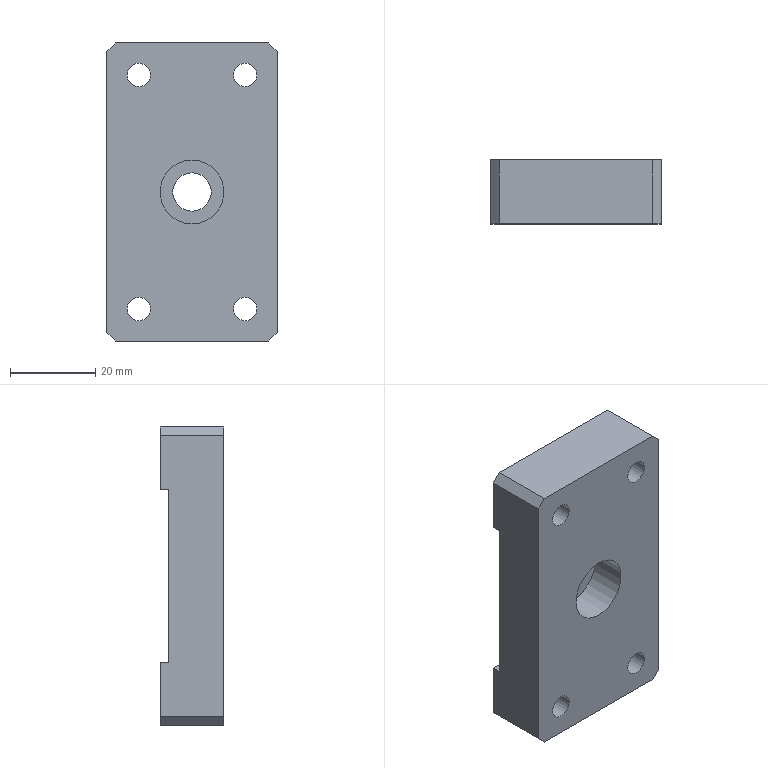Part | NX | 1 solid | 29 faces | box 40 x 15 x 70 mm | volume 34166 mm3 | plane 19 | cylinder 10 | commonest cylinder face diameters 5.5 x4 10 x4 9 x1 15 x1
STEP:
#1=CARTESIAN_POINT('',(-12.5,15.,32.5));
#2=VERTEX_POINT('',#1);
#3=CARTESIAN_POINT('',(-12.5,15.,27.5));
#4=DIRECTION('',(0.,1.,0.));
#5=DIRECTION('',(0.,0.,1.));
#6=AXIS2_PLACEMENT_3D('',#3,#4,#5);
#7=CIRCLE('',#6,5.);
#8=EDGE_CURVE('',#2,#2,#7,.T.);
#9=ORIENTED_EDGE('',*,*,#8,.F.);
#10=EDGE_LOOP('',(#9));
#11=FACE_BOUND('',#10,.T.);
#12=CARTESIAN_POINT('',(12.5,15.,32.5));
#13=VERTEX_POINT('',#12);
#14=CARTESIAN_POINT('',(12.5,15.,27.5));
#15=DIRECTION('',(0.,1.,0.));
#16=DIRECTION('',(0.,0.,1.));
#17=AXIS2_PLACEMENT_3D('',#14,#15,#16);
#18=CIRCLE('',#17,5.);
#19=EDGE_CURVE('',#13,#13,#18,.T.);
#20=ORIENTED_EDGE('',*,*,#19,.F.);
#21=EDGE_LOOP('',(#20));
#22=FACE_BOUND('',#21,.T.);
#23=CARTESIAN_POINT('',(-20.,15.,20.25));
#24=VERTEX_POINT('',#23);
#25=CARTESIAN_POINT('',(-20.,15.,33.));
#26=VERTEX_POINT('',#25);
#27=CARTESIAN_POINT('',(-20.,15.,35.));
#28=DIRECTION('',(0.,0.,1.));
#29=VECTOR('',#28,1000.);
#30=LINE('',#27,#29);
#31=EDGE_CURVE('',#24,#26,#30,.T.);
#32=ORIENTED_EDGE('',*,*,#31,.T.);
#33=CARTESIAN_POINT('',(-18.,15.,35.));
#34=VERTEX_POINT('',#33);
#35=CARTESIAN_POINT('',(-18.,15.,35.));
#36=DIRECTION('',(-0.7071,0.,-0.7071));
#37=VECTOR('',#36,1000.);
#38=LINE('',#35,#37);
#39=EDGE_CURVE('',#26,#34,#38,.F.);
#40=ORIENTED_EDGE('',*,*,#39,.T.);
#41=CARTESIAN_POINT('',(18.,15.,35.));
#42=VERTEX_POINT('',#41);
#43=CARTESIAN_POINT('',(-20.,15.,35.));
#44=DIRECTION('',(1.,0.,0.));
#45=VECTOR('',#44,1000.);
#46=LINE('',#43,#45);
#47=EDGE_CURVE('',#34,#42,#46,.T.);
#48=ORIENTED_EDGE('',*,*,#47,.T.);
#49=CARTESIAN_POINT('',(20.,15.,33.));
#50=VERTEX_POINT('',#49);
#51=CARTESIAN_POINT('',(20.,15.,33.));
#52=DIRECTION('',(-0.7071,0.,0.7071));
#53=VECTOR('',#52,1000.);
#54=LINE('',#51,#53);
#55=EDGE_CURVE('',#42,#50,#54,.F.);
#56=ORIENTED_EDGE('',*,*,#55,.T.);
#57=CARTESIAN_POINT('',(20.,15.,20.25));
#58=VERTEX_POINT('',#57);
#59=CARTESIAN_POINT('',(20.,15.,35.));
#60=DIRECTION('',(0.,0.,-1.));
#61=VECTOR('',#60,1000.);
#62=LINE('',#59,#61);
#63=EDGE_CURVE('',#50,#58,#62,.T.);
#64=ORIENTED_EDGE('',*,*,#63,.T.);
#65=CARTESIAN_POINT('',(-20.25,15.,20.25));
#66=DIRECTION('',(1.,0.,0.));
#67=VECTOR('',#66,1000.);
#68=LINE('',#65,#67);
#69=EDGE_CURVE('',#24,#58,#68,.T.);
#70=ORIENTED_EDGE('',*,*,#69,.F.);
#71=EDGE_LOOP('',(#32,#40,#48,#56,#64,#70));
#72=FACE_BOUND('',#71,.T.);
#73=CARTESIAN_POINT('',(0.,15.,0.));
#74=DIRECTION('',(0.,-1.,0.));
#75=DIRECTION('',(0.,0.,-1.));
#76=AXIS2_PLACEMENT_3D('',#73,#74,#75);
#77=PLANE('',#76);
#78=ADVANCED_FACE('',(#11,#22,#72),#77,.F.);
#79=CARTESIAN_POINT('',(20.,0.,33.));
#80=VERTEX_POINT('',#79);
#81=CARTESIAN_POINT('',(20.,0.,-33.));
#82=VERTEX_POINT('',#81);
#83=CARTESIAN_POINT('',(20.,0.,35.));
#84=DIRECTION('',(0.,0.,-1.));
#85=VECTOR('',#84,1000.);
#86=LINE('',#83,#85);
#87=EDGE_CURVE('',#80,#82,#86,.T.);
#88=ORIENTED_EDGE('',*,*,#87,.T.);
#89=CARTESIAN_POINT('',(20.,15.,-33.));
#90=VERTEX_POINT('',#89);
#91=CARTESIAN_POINT('',(20.,15.,-33.));
#92=DIRECTION('',(0.,1.,0.));
#93=VECTOR('',#92,1000.);
#94=LINE('',#91,#93);
#95=EDGE_CURVE('',#82,#90,#94,.T.);
#96=ORIENTED_EDGE('',*,*,#95,.T.);
#97=CARTESIAN_POINT('',(20.,15.,-20.25));
#98=VERTEX_POINT('',#97);
#99=CARTESIAN_POINT('',(20.,15.,35.));
#100=DIRECTION('',(0.,0.,-1.));
#101=VECTOR('',#100,1000.);
#102=LINE('',#99,#101);
#103=EDGE_CURVE('',#98,#90,#102,.T.);
#104=ORIENTED_EDGE('',*,*,#103,.F.);
#105=CARTESIAN_POINT('',(20.,13.,-20.25));
#106=VERTEX_POINT('',#105);
#107=CARTESIAN_POINT('',(20.,15.,-20.25));
#108=DIRECTION('',(0.,-1.,0.));
#109=VECTOR('',#108,1000.);
#110=LINE('',#107,#109);
#111=EDGE_CURVE('',#98,#106,#110,.T.);
#112=ORIENTED_EDGE('',*,*,#111,.T.);
#113=CARTESIAN_POINT('',(20.,13.,20.25));
#114=VERTEX_POINT('',#113);
#115=CARTESIAN_POINT('',(20.,13.,35.));
#116=DIRECTION('',(0.,0.,1.));
#117=VECTOR('',#116,1000.);
#118=LINE('',#115,#117);
#119=EDGE_CURVE('',#106,#114,#118,.T.);
#120=ORIENTED_EDGE('',*,*,#119,.T.);
#121=CARTESIAN_POINT('',(20.,15.,20.25));
#122=DIRECTION('',(0.,1.,0.));
#123=VECTOR('',#122,1000.);
#124=LINE('',#121,#123);
#125=EDGE_CURVE('',#114,#58,#124,.T.);
#126=ORIENTED_EDGE('',*,*,#125,.T.);
#127=ORIENTED_EDGE('',*,*,#63,.F.);
#128=CARTESIAN_POINT('',(20.,15.,33.));
#129=DIRECTION('',(0.,-1.,0.));
#130=VECTOR('',#129,1000.);
#131=LINE('',#128,#130);
#132=EDGE_CURVE('',#50,#80,#131,.T.);
#133=ORIENTED_EDGE('',*,*,#132,.T.);
#134=EDGE_LOOP('',(#88,#96,#104,#112,#120,#126,#127,#133));
#135=FACE_BOUND('',#134,.T.);
#136=CARTESIAN_POINT('',(20.,15.,35.));
#137=DIRECTION('',(-1.,0.,0.));
#138=DIRECTION('',(0.,0.,1.));
#139=AXIS2_PLACEMENT_3D('',#136,#137,#138);
#140=PLANE('',#139);
#141=ADVANCED_FACE('',(#135),#140,.F.);
#142=CARTESIAN_POINT('',(18.,15.,-35.));
#143=VERTEX_POINT('',#142);
#144=CARTESIAN_POINT('',(-18.,15.,-35.));
#145=VERTEX_POINT('',#144);
#146=CARTESIAN_POINT('',(-20.,15.,-35.));
#147=DIRECTION('',(-1.,0.,0.));
#148=VECTOR('',#147,1000.);
#149=LINE('',#146,#148);
#150=EDGE_CURVE('',#143,#145,#149,.T.);
#151=ORIENTED_EDGE('',*,*,#150,.F.);
#152=CARTESIAN_POINT('',(18.,0.,-35.));
#153=VERTEX_POINT('',#152);
#154=CARTESIAN_POINT('',(18.,15.,-35.));
#155=DIRECTION('',(0.,-1.,0.));
#156=VECTOR('',#155,1000.);
#157=LINE('',#154,#156);
#158=EDGE_CURVE('',#143,#153,#157,.T.);
#159=ORIENTED_EDGE('',*,*,#158,.T.);
#160=CARTESIAN_POINT('',(-18.,0.,-35.));
#161=VERTEX_POINT('',#160);
#162=CARTESIAN_POINT('',(-20.,0.,-35.));
#163=DIRECTION('',(-1.,0.,0.));
#164=VECTOR('',#163,1000.);
#165=LINE('',#162,#164);
#166=EDGE_CURVE('',#153,#161,#165,.T.);
#167=ORIENTED_EDGE('',*,*,#166,.T.);
#168=CARTESIAN_POINT('',(-18.,15.,-35.));
#169=DIRECTION('',(0.,1.,0.));
#170=VECTOR('',#169,1000.);
#171=LINE('',#168,#170);
#172=EDGE_CURVE('',#161,#145,#171,.T.);
#173=ORIENTED_EDGE('',*,*,#172,.T.);
#174=EDGE_LOOP('',(#151,#159,#167,#173));
#175=FACE_BOUND('',#174,.T.);
#176=CARTESIAN_POINT('',(-20.,15.,-35.));
#177=DIRECTION('',(0.,0.,1.));
#178=DIRECTION('',(1.,0.,0.));
#179=AXIS2_PLACEMENT_3D('',#176,#177,#178);
#180=PLANE('',#179);
#181=ADVANCED_FACE('',(#175),#180,.F.);
#182=CARTESIAN_POINT('',(-20.,15.,-33.));
#183=VERTEX_POINT('',#182);
#184=CARTESIAN_POINT('',(-20.,15.,-20.25));
#185=VERTEX_POINT('',#184);
#186=CARTESIAN_POINT('',(-20.,15.,35.));
#187=DIRECTION('',(0.,0.,1.));
#188=VECTOR('',#187,1000.);
#189=LINE('',#186,#188);
#190=EDGE_CURVE('',#183,#185,#189,.T.);
#191=ORIENTED_EDGE('',*,*,#190,.F.);
#192=CARTESIAN_POINT('',(-20.,0.,-33.));
#193=VERTEX_POINT('',#192);
#194=CARTESIAN_POINT('',(-20.,15.,-33.));
#195=DIRECTION('',(0.,-1.,0.));
#196=VECTOR('',#195,1000.);
#197=LINE('',#194,#196);
#198=EDGE_CURVE('',#183,#193,#197,.T.);
#199=ORIENTED_EDGE('',*,*,#198,.T.);
#200=CARTESIAN_POINT('',(-20.,0.,33.));
#201=VERTEX_POINT('',#200);
#202=CARTESIAN_POINT('',(-20.,0.,35.));
#203=DIRECTION('',(0.,0.,1.));
#204=VECTOR('',#203,1000.);
#205=LINE('',#202,#204);
#206=EDGE_CURVE('',#193,#201,#205,.T.);
#207=ORIENTED_EDGE('',*,*,#206,.T.);
#208=CARTESIAN_POINT('',(-20.,15.,33.));
#209=DIRECTION('',(0.,1.,0.));
#210=VECTOR('',#209,1000.);
#211=LINE('',#208,#210);
#212=EDGE_CURVE('',#201,#26,#211,.T.);
#213=ORIENTED_EDGE('',*,*,#212,.T.);
#214=ORIENTED_EDGE('',*,*,#31,.F.);
#215=CARTESIAN_POINT('',(-20.,13.,20.25));
#216=VERTEX_POINT('',#215);
#217=CARTESIAN_POINT('',(-20.,15.,20.25));
#218=DIRECTION('',(0.,-1.,0.));
#219=VECTOR('',#218,1000.);
#220=LINE('',#217,#219);
#221=EDGE_CURVE('',#24,#216,#220,.T.);
#222=ORIENTED_EDGE('',*,*,#221,.T.);
#223=CARTESIAN_POINT('',(-20.,13.,-20.25));
#224=VERTEX_POINT('',#223);
#225=CARTESIAN_POINT('',(-20.,13.,35.));
#226=DIRECTION('',(0.,0.,-1.));
#227=VECTOR('',#226,1000.);
#228=LINE('',#225,#227);
#229=EDGE_CURVE('',#216,#224,#228,.T.);
#230=ORIENTED_EDGE('',*,*,#229,.T.);
#231=CARTESIAN_POINT('',(-20.,15.,-20.25));
#232=DIRECTION('',(0.,1.,0.));
#233=VECTOR('',#232,1000.);
#234=LINE('',#231,#233);
#235=EDGE_CURVE('',#224,#185,#234,.T.);
#236=ORIENTED_EDGE('',*,*,#235,.T.);
#237=EDGE_LOOP('',(#191,#199,#207,#213,#214,#222,#230,#236));
#238=FACE_BOUND('',#237,.T.);
#239=CARTESIAN_POINT('',(-20.,15.,35.));
#240=DIRECTION('',(1.,0.,0.));
#241=DIRECTION('',(0.,0.,-1.));
#242=AXIS2_PLACEMENT_3D('',#239,#240,#241);
#243=PLANE('',#242);
#244=ADVANCED_FACE('',(#238),#243,.F.);
#245=ORIENTED_EDGE('',*,*,#47,.F.);
#246=CARTESIAN_POINT('',(-18.,0.,35.));
#247=VERTEX_POINT('',#246);
#248=CARTESIAN_POINT('',(-18.,15.,35.));
#249=DIRECTION('',(0.,-1.,0.));
#250=VECTOR('',#249,1000.);
#251=LINE('',#248,#250);
#252=EDGE_CURVE('',#34,#247,#251,.T.);
#253=ORIENTED_EDGE('',*,*,#252,.T.);
#254=CARTESIAN_POINT('',(18.,0.,35.));
#255=VERTEX_POINT('',#254);
#256=CARTESIAN_POINT('',(-20.,0.,35.));
#257=DIRECTION('',(1.,0.,0.));
#258=VECTOR('',#257,1000.);
#259=LINE('',#256,#258);
#260=EDGE_CURVE('',#247,#255,#259,.T.);
#261=ORIENTED_EDGE('',*,*,#260,.T.);
#262=CARTESIAN_POINT('',(18.,15.,35.));
#263=DIRECTION('',(0.,1.,0.));
#264=VECTOR('',#263,1000.);
#265=LINE('',#262,#264);
#266=EDGE_CURVE('',#255,#42,#265,.T.);
#267=ORIENTED_EDGE('',*,*,#266,.T.);
#268=EDGE_LOOP('',(#245,#253,#261,#267));
#269=FACE_BOUND('',#268,.T.);
#270=CARTESIAN_POINT('',(-20.,15.,35.));
#271=DIRECTION('',(0.,0.,-1.));
#272=DIRECTION('',(-1.,0.,0.));
#273=AXIS2_PLACEMENT_3D('',#270,#271,#272);
#274=PLANE('',#273);
#275=ADVANCED_FACE('',(#269),#274,.F.);
#276=CARTESIAN_POINT('',(-12.5,15.,-22.5));
#277=VERTEX_POINT('',#276);
#278=CARTESIAN_POINT('',(-12.5,15.,-27.5));
#279=DIRECTION('',(0.,1.,0.));
#280=DIRECTION('',(0.,0.,1.));
#281=AXIS2_PLACEMENT_3D('',#278,#279,#280);
#282=CIRCLE('',#281,5.);
#283=EDGE_CURVE('',#277,#277,#282,.T.);
#284=ORIENTED_EDGE('',*,*,#283,.F.);
#285=EDGE_LOOP('',(#284));
#286=FACE_BOUND('',#285,.T.);
#287=CARTESIAN_POINT('',(12.5,15.,-22.5));
#288=VERTEX_POINT('',#287);
#289=CARTESIAN_POINT('',(12.5,15.,-27.5));
#290=DIRECTION('',(0.,1.,0.));
#291=DIRECTION('',(0.,0.,1.));
#292=AXIS2_PLACEMENT_3D('',#289,#290,#291);
#293=CIRCLE('',#292,5.);
#294=EDGE_CURVE('',#288,#288,#293,.T.);
#295=ORIENTED_EDGE('',*,*,#294,.F.);
#296=EDGE_LOOP('',(#295));
#297=FACE_BOUND('',#296,.T.);
#298=ORIENTED_EDGE('',*,*,#103,.T.);
#299=CARTESIAN_POINT('',(18.,15.,-35.));
#300=DIRECTION('',(0.7071,0.,0.7071));
#301=VECTOR('',#300,1000.);
#302=LINE('',#299,#301);
#303=EDGE_CURVE('',#90,#143,#302,.F.);
#304=ORIENTED_EDGE('',*,*,#303,.T.);
#305=ORIENTED_EDGE('',*,*,#150,.T.);
#306=CARTESIAN_POINT('',(-20.,15.,-33.));
#307=DIRECTION('',(0.7071,0.,-0.7071));
#308=VECTOR('',#307,1000.);
#309=LINE('',#306,#308);
#310=EDGE_CURVE('',#145,#183,#309,.F.);
#311=ORIENTED_EDGE('',*,*,#310,.T.);
#312=ORIENTED_EDGE('',*,*,#190,.T.);
#313=CARTESIAN_POINT('',(-20.25,15.,-20.25));
#314=DIRECTION('',(-1.,0.,0.));
#315=VECTOR('',#314,1000.);
#316=LINE('',#313,#315);
#317=EDGE_CURVE('',#98,#185,#316,.T.);
#318=ORIENTED_EDGE('',*,*,#317,.F.);
#319=EDGE_LOOP('',(#298,#304,#305,#311,#312,#318));
#320=FACE_BOUND('',#319,.T.);
#321=CARTESIAN_POINT('',(0.,15.,0.));
#322=DIRECTION('',(0.,-1.,0.));
#323=DIRECTION('',(0.,0.,-1.));
#324=AXIS2_PLACEMENT_3D('',#321,#322,#323);
#325=PLANE('',#324);
#326=ADVANCED_FACE('',(#286,#297,#320),#325,.F.);
#327=CARTESIAN_POINT('',(0.,0.,-7.5));
#328=VERTEX_POINT('',#327);
#329=CARTESIAN_POINT('',(0.,0.,0.));
#330=DIRECTION('',(0.,-1.,0.));
#331=DIRECTION('',(0.,0.,-1.));
#332=AXIS2_PLACEMENT_3D('',#329,#330,#331);
#333=CIRCLE('',#332,7.5);
#334=EDGE_CURVE('',#328,#328,#333,.T.);
#335=ORIENTED_EDGE('',*,*,#334,.F.);
#336=EDGE_LOOP('',(#335));
#337=FACE_BOUND('',#336,.T.);
#338=CARTESIAN_POINT('',(-12.5,0.,-24.75));
#339=VERTEX_POINT('',#338);
#340=CARTESIAN_POINT('',(-12.5,0.,-27.5));
#341=DIRECTION('',(0.,1.,0.));
#342=DIRECTION('',(0.,0.,1.));
#343=AXIS2_PLACEMENT_3D('',#340,#341,#342);
#344=CIRCLE('',#343,2.75);
#345=EDGE_CURVE('',#339,#339,#344,.T.);
#346=ORIENTED_EDGE('',*,*,#345,.T.);
#347=EDGE_LOOP('',(#346));
#348=FACE_BOUND('',#347,.T.);
#349=CARTESIAN_POINT('',(12.5,0.,-24.75));
#350=VERTEX_POINT('',#349);
#351=CARTESIAN_POINT('',(12.5,0.,-27.5));
#352=DIRECTION('',(0.,1.,0.));
#353=DIRECTION('',(0.,0.,1.));
#354=AXIS2_PLACEMENT_3D('',#351,#352,#353);
#355=CIRCLE('',#354,2.75);
#356=EDGE_CURVE('',#350,#350,#355,.T.);
#357=ORIENTED_EDGE('',*,*,#356,.T.);
#358=EDGE_LOOP('',(#357));
#359=FACE_BOUND('',#358,.T.);
#360=CARTESIAN_POINT('',(12.5,0.,30.25));
#361=VERTEX_POINT('',#360);
#362=CARTESIAN_POINT('',(12.5,0.,27.5));
#363=DIRECTION('',(0.,1.,0.));
#364=DIRECTION('',(0.,0.,1.));
#365=AXIS2_PLACEMENT_3D('',#362,#363,#364);
#366=CIRCLE('',#365,2.75);
#367=EDGE_CURVE('',#361,#361,#366,.T.);
#368=ORIENTED_EDGE('',*,*,#367,.T.);
#369=EDGE_LOOP('',(#368));
#370=FACE_BOUND('',#369,.T.);
#371=CARTESIAN_POINT('',(-12.5,0.,30.25));
#372=VERTEX_POINT('',#371);
#373=CARTESIAN_POINT('',(-12.5,0.,27.5));
#374=DIRECTION('',(0.,1.,0.));
#375=DIRECTION('',(0.,0.,1.));
#376=AXIS2_PLACEMENT_3D('',#373,#374,#375);
#377=CIRCLE('',#376,2.75);
#378=EDGE_CURVE('',#372,#372,#377,.T.);
#379=ORIENTED_EDGE('',*,*,#378,.T.);
#380=EDGE_LOOP('',(#379));
#381=FACE_BOUND('',#380,.T.);
#382=ORIENTED_EDGE('',*,*,#166,.F.);
#383=CARTESIAN_POINT('',(26.5,0.,-26.5));
#384=DIRECTION('',(-0.7071,0.,-0.7071));
#385=VECTOR('',#384,1000.);
#386=LINE('',#383,#385);
#387=EDGE_CURVE('',#153,#82,#386,.F.);
#388=ORIENTED_EDGE('',*,*,#387,.T.);
#389=ORIENTED_EDGE('',*,*,#87,.F.);
#390=CARTESIAN_POINT('',(26.5,0.,26.5));
#391=DIRECTION('',(0.7071,0.,-0.7071));
#392=VECTOR('',#391,1000.);
#393=LINE('',#390,#392);
#394=EDGE_CURVE('',#80,#255,#393,.F.);
#395=ORIENTED_EDGE('',*,*,#394,.T.);
#396=ORIENTED_EDGE('',*,*,#260,.F.);
#397=CARTESIAN_POINT('',(-26.5,0.,26.5));
#398=DIRECTION('',(0.7071,0.,0.7071));
#399=VECTOR('',#398,1000.);
#400=LINE('',#397,#399);
#401=EDGE_CURVE('',#247,#201,#400,.F.);
#402=ORIENTED_EDGE('',*,*,#401,.T.);
#403=ORIENTED_EDGE('',*,*,#206,.F.);
#404=CARTESIAN_POINT('',(-26.5,0.,-26.5));
#405=DIRECTION('',(-0.7071,0.,0.7071));
#406=VECTOR('',#405,1000.);
#407=LINE('',#404,#406);
#408=EDGE_CURVE('',#193,#161,#407,.F.);
#409=ORIENTED_EDGE('',*,*,#408,.T.);
#410=EDGE_LOOP('',(#382,#388,#389,#395,#396,#402,#403,#409));
#411=FACE_BOUND('',#410,.T.);
#412=CARTESIAN_POINT('',(0.,0.,0.));
#413=DIRECTION('',(0.,-1.,0.));
#414=DIRECTION('',(0.,0.,-1.));
#415=AXIS2_PLACEMENT_3D('',#412,#413,#414);
#416=PLANE('',#415);
#417=ADVANCED_FACE('',(#337,#348,#359,#370,#381,#411),#416,.T.);
#418=ORIENTED_EDGE('',*,*,#378,.F.);
#419=EDGE_LOOP('',(#418));
#420=FACE_BOUND('',#419,.T.);
#421=CARTESIAN_POINT('',(-12.5,9.3,30.25));
#422=VERTEX_POINT('',#421);
#423=CARTESIAN_POINT('',(-12.5,9.3,27.5));
#424=DIRECTION('',(0.,1.,0.));
#425=DIRECTION('',(0.,0.,1.));
#426=AXIS2_PLACEMENT_3D('',#423,#424,#425);
#427=CIRCLE('',#426,2.75);
#428=EDGE_CURVE('',#422,#422,#427,.T.);
#429=ORIENTED_EDGE('',*,*,#428,.T.);
#430=EDGE_LOOP('',(#429));
#431=FACE_BOUND('',#430,.T.);
#432=CARTESIAN_POINT('',(-12.5,15.,27.5));
#433=DIRECTION('',(0.,1.,0.));
#434=DIRECTION('',(0.,0.,1.));
#435=AXIS2_PLACEMENT_3D('',#432,#433,#434);
#436=CYLINDRICAL_SURFACE('',#435,2.75);
#437=ADVANCED_FACE('',(#420,#431),#436,.F.);
#438=ORIENTED_EDGE('',*,*,#428,.F.);
#439=EDGE_LOOP('',(#438));
#440=FACE_BOUND('',#439,.T.);
#441=CARTESIAN_POINT('',(-12.5,9.3,32.5));
#442=VERTEX_POINT('',#441);
#443=CARTESIAN_POINT('',(-12.5,9.3,27.5));
#444=DIRECTION('',(0.,1.,0.));
#445=DIRECTION('',(0.,0.,1.));
#446=AXIS2_PLACEMENT_3D('',#443,#444,#445);
#447=CIRCLE('',#446,5.);
#448=EDGE_CURVE('',#442,#442,#447,.T.);
#449=ORIENTED_EDGE('',*,*,#448,.T.);
#450=EDGE_LOOP('',(#449));
#451=FACE_BOUND('',#450,.T.);
#452=CARTESIAN_POINT('',(-9.75,9.3,27.5));
#453=DIRECTION('',(0.,-1.,0.));
#454=DIRECTION('',(0.,0.,-1.));
#455=AXIS2_PLACEMENT_3D('',#452,#453,#454);
#456=PLANE('',#455);
#457=ADVANCED_FACE('',(#440,#451),#456,.F.);
#458=ORIENTED_EDGE('',*,*,#448,.F.);
#459=EDGE_LOOP('',(#458));
#460=FACE_BOUND('',#459,.T.);
#461=ORIENTED_EDGE('',*,*,#8,.T.);
#462=EDGE_LOOP('',(#461));
#463=FACE_BOUND('',#462,.T.);
#464=CARTESIAN_POINT('',(-12.5,15.,27.5));
#465=DIRECTION('',(0.,1.,0.));
#466=DIRECTION('',(0.,0.,1.));
#467=AXIS2_PLACEMENT_3D('',#464,#465,#466);
#468=CYLINDRICAL_SURFACE('',#467,5.);
#469=ADVANCED_FACE('',(#460,#463),#468,.F.);
#470=ORIENTED_EDGE('',*,*,#367,.F.);
#471=EDGE_LOOP('',(#470));
#472=FACE_BOUND('',#471,.T.);
#473=CARTESIAN_POINT('',(12.5,9.3,30.25));
#474=VERTEX_POINT('',#473);
#475=CARTESIAN_POINT('',(12.5,9.3,27.5));
#476=DIRECTION('',(0.,1.,0.));
#477=DIRECTION('',(0.,0.,1.));
#478=AXIS2_PLACEMENT_3D('',#475,#476,#477);
#479=CIRCLE('',#478,2.75);
#480=EDGE_CURVE('',#474,#474,#479,.T.);
#481=ORIENTED_EDGE('',*,*,#480,.T.);
#482=EDGE_LOOP('',(#481));
#483=FACE_BOUND('',#482,.T.);
#484=CARTESIAN_POINT('',(12.5,15.,27.5));
#485=DIRECTION('',(0.,1.,0.));
#486=DIRECTION('',(0.,0.,1.));
#487=AXIS2_PLACEMENT_3D('',#484,#485,#486);
#488=CYLINDRICAL_SURFACE('',#487,2.75);
#489=ADVANCED_FACE('',(#472,#483),#488,.F.);
#490=ORIENTED_EDGE('',*,*,#480,.F.);
#491=EDGE_LOOP('',(#490));
#492=FACE_BOUND('',#491,.T.);
#493=CARTESIAN_POINT('',(12.5,9.3,32.5));
#494=VERTEX_POINT('',#493);
#495=CARTESIAN_POINT('',(12.5,9.3,27.5));
#496=DIRECTION('',(0.,1.,0.));
#497=DIRECTION('',(0.,0.,1.));
#498=AXIS2_PLACEMENT_3D('',#495,#496,#497);
#499=CIRCLE('',#498,5.);
#500=EDGE_CURVE('',#494,#494,#499,.T.);
#501=ORIENTED_EDGE('',*,*,#500,.T.);
#502=EDGE_LOOP('',(#501));
#503=FACE_BOUND('',#502,.T.);
#504=CARTESIAN_POINT('',(15.25,9.3,27.5));
#505=DIRECTION('',(0.,-1.,0.));
#506=DIRECTION('',(0.,0.,-1.));
#507=AXIS2_PLACEMENT_3D('',#504,#505,#506);
#508=PLANE('',#507);
#509=ADVANCED_FACE('',(#492,#503),#508,.F.);
#510=ORIENTED_EDGE('',*,*,#500,.F.);
#511=EDGE_LOOP('',(#510));
#512=FACE_BOUND('',#511,.T.);
#513=ORIENTED_EDGE('',*,*,#19,.T.);
#514=EDGE_LOOP('',(#513));
#515=FACE_BOUND('',#514,.T.);
#516=CARTESIAN_POINT('',(12.5,15.,27.5));
#517=DIRECTION('',(0.,1.,0.));
#518=DIRECTION('',(0.,0.,1.));
#519=AXIS2_PLACEMENT_3D('',#516,#517,#518);
#520=CYLINDRICAL_SURFACE('',#519,5.);
#521=ADVANCED_FACE('',(#512,#515),#520,.F.);
#522=ORIENTED_EDGE('',*,*,#356,.F.);
#523=EDGE_LOOP('',(#522));
#524=FACE_BOUND('',#523,.T.);
#525=CARTESIAN_POINT('',(12.5,9.3,-24.75));
#526=VERTEX_POINT('',#525);
#527=CARTESIAN_POINT('',(12.5,9.3,-27.5));
#528=DIRECTION('',(0.,1.,0.));
#529=DIRECTION('',(0.,0.,1.));
#530=AXIS2_PLACEMENT_3D('',#527,#528,#529);
#531=CIRCLE('',#530,2.75);
#532=EDGE_CURVE('',#526,#526,#531,.T.);
#533=ORIENTED_EDGE('',*,*,#532,.T.);
#534=EDGE_LOOP('',(#533));
#535=FACE_BOUND('',#534,.T.);
#536=CARTESIAN_POINT('',(12.5,15.,-27.5));
#537=DIRECTION('',(0.,1.,0.));
#538=DIRECTION('',(0.,0.,1.));
#539=AXIS2_PLACEMENT_3D('',#536,#537,#538);
#540=CYLINDRICAL_SURFACE('',#539,2.75);
#541=ADVANCED_FACE('',(#524,#535),#540,.F.);
#542=ORIENTED_EDGE('',*,*,#532,.F.);
#543=EDGE_LOOP('',(#542));
#544=FACE_BOUND('',#543,.T.);
#545=CARTESIAN_POINT('',(12.5,9.3,-22.5));
#546=VERTEX_POINT('',#545);
#547=CARTESIAN_POINT('',(12.5,9.3,-27.5));
#548=DIRECTION('',(0.,1.,0.));
#549=DIRECTION('',(0.,0.,1.));
#550=AXIS2_PLACEMENT_3D('',#547,#548,#549);
#551=CIRCLE('',#550,5.);
#552=EDGE_CURVE('',#546,#546,#551,.T.);
#553=ORIENTED_EDGE('',*,*,#552,.T.);
#554=EDGE_LOOP('',(#553));
#555=FACE_BOUND('',#554,.T.);
#556=CARTESIAN_POINT('',(15.25,9.3,-27.5));
#557=DIRECTION('',(0.,-1.,0.));
#558=DIRECTION('',(0.,0.,-1.));
#559=AXIS2_PLACEMENT_3D('',#556,#557,#558);
#560=PLANE('',#559);
#561=ADVANCED_FACE('',(#544,#555),#560,.F.);
#562=ORIENTED_EDGE('',*,*,#552,.F.);
#563=EDGE_LOOP('',(#562));
#564=FACE_BOUND('',#563,.T.);
#565=ORIENTED_EDGE('',*,*,#294,.T.);
#566=EDGE_LOOP('',(#565));
#567=FACE_BOUND('',#566,.T.);
#568=CARTESIAN_POINT('',(12.5,15.,-27.5));
#569=DIRECTION('',(0.,1.,0.));
#570=DIRECTION('',(0.,0.,1.));
#571=AXIS2_PLACEMENT_3D('',#568,#569,#570);
#572=CYLINDRICAL_SURFACE('',#571,5.);
#573=ADVANCED_FACE('',(#564,#567),#572,.F.);
#574=ORIENTED_EDGE('',*,*,#345,.F.);
#575=EDGE_LOOP('',(#574));
#576=FACE_BOUND('',#575,.T.);
#577=CARTESIAN_POINT('',(-12.5,9.3,-24.75));
#578=VERTEX_POINT('',#577);
#579=CARTESIAN_POINT('',(-12.5,9.3,-27.5));
#580=DIRECTION('',(0.,1.,0.));
#581=DIRECTION('',(0.,0.,1.));
#582=AXIS2_PLACEMENT_3D('',#579,#580,#581);
#583=CIRCLE('',#582,2.75);
#584=EDGE_CURVE('',#578,#578,#583,.T.);
#585=ORIENTED_EDGE('',*,*,#584,.T.);
#586=EDGE_LOOP('',(#585));
#587=FACE_BOUND('',#586,.T.);
#588=CARTESIAN_POINT('',(-12.5,15.,-27.5));
#589=DIRECTION('',(0.,1.,0.));
#590=DIRECTION('',(0.,0.,1.));
#591=AXIS2_PLACEMENT_3D('',#588,#589,#590);
#592=CYLINDRICAL_SURFACE('',#591,2.75);
#593=ADVANCED_FACE('',(#576,#587),#592,.F.);
#594=ORIENTED_EDGE('',*,*,#584,.F.);
#595=EDGE_LOOP('',(#594));
#596=FACE_BOUND('',#595,.T.);
#597=CARTESIAN_POINT('',(-12.5,9.3,-22.5));
#598=VERTEX_POINT('',#597);
#599=CARTESIAN_POINT('',(-12.5,9.3,-27.5));
#600=DIRECTION('',(0.,1.,0.));
#601=DIRECTION('',(0.,0.,1.));
#602=AXIS2_PLACEMENT_3D('',#599,#600,#601);
#603=CIRCLE('',#602,5.);
#604=EDGE_CURVE('',#598,#598,#603,.T.);
#605=ORIENTED_EDGE('',*,*,#604,.T.);
#606=EDGE_LOOP('',(#605));
#607=FACE_BOUND('',#606,.T.);
#608=CARTESIAN_POINT('',(-9.75,9.3,-27.5));
#609=DIRECTION('',(0.,-1.,0.));
#610=DIRECTION('',(0.,0.,-1.));
#611=AXIS2_PLACEMENT_3D('',#608,#609,#610);
#612=PLANE('',#611);
#613=ADVANCED_FACE('',(#596,#607),#612,.F.);
#614=ORIENTED_EDGE('',*,*,#604,.F.);
#615=EDGE_LOOP('',(#614));
#616=FACE_BOUND('',#615,.T.);
#617=ORIENTED_EDGE('',*,*,#283,.T.);
#618=EDGE_LOOP('',(#617));
#619=FACE_BOUND('',#618,.T.);
#620=CARTESIAN_POINT('',(-12.5,15.,-27.5));
#621=DIRECTION('',(0.,1.,0.));
#622=DIRECTION('',(0.,0.,1.));
#623=AXIS2_PLACEMENT_3D('',#620,#621,#622);
#624=CYLINDRICAL_SURFACE('',#623,5.);
#625=ADVANCED_FACE('',(#616,#619),#624,.F.);
#626=CARTESIAN_POINT('',(0.,13.,-4.5));
#627=VERTEX_POINT('',#626);
#628=CARTESIAN_POINT('',(0.,13.,0.));
#629=DIRECTION('',(0.,-1.,0.));
#630=DIRECTION('',(0.,0.,-1.));
#631=AXIS2_PLACEMENT_3D('',#628,#629,#630);
#632=CIRCLE('',#631,4.5);
#633=EDGE_CURVE('',#627,#627,#632,.F.);
#634=ORIENTED_EDGE('',*,*,#633,.T.);
#635=EDGE_LOOP('',(#634));
#636=FACE_BOUND('',#635,.T.);
#637=CARTESIAN_POINT('',(0.,8.6,-4.5));
#638=VERTEX_POINT('',#637);
#639=CARTESIAN_POINT('',(0.,8.6,0.));
#640=DIRECTION('',(0.,-1.,0.));
#641=DIRECTION('',(0.,0.,-1.));
#642=AXIS2_PLACEMENT_3D('',#639,#640,#641);
#643=CIRCLE('',#642,4.5);
#644=EDGE_CURVE('',#638,#638,#643,.T.);
#645=ORIENTED_EDGE('',*,*,#644,.T.);
#646=EDGE_LOOP('',(#645));
#647=FACE_BOUND('',#646,.T.);
#648=CARTESIAN_POINT('',(0.,0.,0.));
#649=DIRECTION('',(0.,-1.,0.));
#650=DIRECTION('',(0.,0.,-1.));
#651=AXIS2_PLACEMENT_3D('',#648,#649,#650);
#652=CYLINDRICAL_SURFACE('',#651,4.5);
#653=ADVANCED_FACE('',(#636,#647),#652,.F.);
#654=ORIENTED_EDGE('',*,*,#644,.F.);
#655=EDGE_LOOP('',(#654));
#656=FACE_BOUND('',#655,.T.);
#657=CARTESIAN_POINT('',(0.,8.6,-7.5));
#658=VERTEX_POINT('',#657);
#659=CARTESIAN_POINT('',(0.,8.6,0.));
#660=DIRECTION('',(0.,-1.,0.));
#661=DIRECTION('',(0.,0.,-1.));
#662=AXIS2_PLACEMENT_3D('',#659,#660,#661);
#663=CIRCLE('',#662,7.5);
#664=EDGE_CURVE('',#658,#658,#663,.T.);
#665=ORIENTED_EDGE('',*,*,#664,.T.);
#666=EDGE_LOOP('',(#665));
#667=FACE_BOUND('',#666,.T.);
#668=CARTESIAN_POINT('',(4.5,8.6,0.));
#669=DIRECTION('',(0.,1.,0.));
#670=DIRECTION('',(0.,0.,1.));
#671=AXIS2_PLACEMENT_3D('',#668,#669,#670);
#672=PLANE('',#671);
#673=ADVANCED_FACE('',(#656,#667),#672,.F.);
#674=ORIENTED_EDGE('',*,*,#664,.F.);
#675=EDGE_LOOP('',(#674));
#676=FACE_BOUND('',#675,.T.);
#677=ORIENTED_EDGE('',*,*,#334,.T.);
#678=EDGE_LOOP('',(#677));
#679=FACE_BOUND('',#678,.T.);
#680=CARTESIAN_POINT('',(0.,0.,0.));
#681=DIRECTION('',(0.,-1.,0.));
#682=DIRECTION('',(0.,0.,-1.));
#683=AXIS2_PLACEMENT_3D('',#680,#681,#682);
#684=CYLINDRICAL_SURFACE('',#683,7.5);
#685=ADVANCED_FACE('',(#676,#679),#684,.F.);
#686=CARTESIAN_POINT('',(-20.25,13.,20.25));
#687=DIRECTION('',(1.,0.,0.));
#688=VECTOR('',#687,1000.);
#689=LINE('',#686,#688);
#690=EDGE_CURVE('',#216,#114,#689,.T.);
#691=ORIENTED_EDGE('',*,*,#690,.F.);
#692=ORIENTED_EDGE('',*,*,#221,.F.);
#693=ORIENTED_EDGE('',*,*,#69,.T.);
#694=ORIENTED_EDGE('',*,*,#125,.F.);
#695=EDGE_LOOP('',(#691,#692,#693,#694));
#696=FACE_BOUND('',#695,.T.);
#697=CARTESIAN_POINT('',(-20.25,13.,20.25));
#698=DIRECTION('',(0.,0.,1.));
#699=DIRECTION('',(1.,0.,0.));
#700=AXIS2_PLACEMENT_3D('',#697,#698,#699);
#701=PLANE('',#700);
#702=ADVANCED_FACE('',(#696),#701,.F.);
#703=ORIENTED_EDGE('',*,*,#317,.T.);
#704=ORIENTED_EDGE('',*,*,#235,.F.);
#705=CARTESIAN_POINT('',(-20.25,13.,-20.25));
#706=DIRECTION('',(-1.,0.,0.));
#707=VECTOR('',#706,1000.);
#708=LINE('',#705,#707);
#709=EDGE_CURVE('',#106,#224,#708,.T.);
#710=ORIENTED_EDGE('',*,*,#709,.F.);
#711=ORIENTED_EDGE('',*,*,#111,.F.);
#712=EDGE_LOOP('',(#703,#704,#710,#711));
#713=FACE_BOUND('',#712,.T.);
#714=CARTESIAN_POINT('',(-20.25,13.,-20.25));
#715=DIRECTION('',(0.,0.,-1.));
#716=DIRECTION('',(-1.,0.,0.));
#717=AXIS2_PLACEMENT_3D('',#714,#715,#716);
#718=PLANE('',#717);
#719=ADVANCED_FACE('',(#713),#718,.F.);
#720=ORIENTED_EDGE('',*,*,#633,.F.);
#721=EDGE_LOOP('',(#720));
#722=FACE_BOUND('',#721,.T.);
#723=ORIENTED_EDGE('',*,*,#709,.T.);
#724=ORIENTED_EDGE('',*,*,#229,.F.);
#725=ORIENTED_EDGE('',*,*,#690,.T.);
#726=ORIENTED_EDGE('',*,*,#119,.F.);
#727=EDGE_LOOP('',(#723,#724,#725,#726));
#728=FACE_BOUND('',#727,.T.);
#729=CARTESIAN_POINT('',(0.,13.,0.));
#730=DIRECTION('',(0.,-1.,0.));
#731=DIRECTION('',(0.,0.,-1.));
#732=AXIS2_PLACEMENT_3D('',#729,#730,#731);
#733=PLANE('',#732);
#734=ADVANCED_FACE('',(#722,#728),#733,.F.);
#735=ORIENTED_EDGE('',*,*,#303,.F.);
#736=ORIENTED_EDGE('',*,*,#95,.F.);
#737=ORIENTED_EDGE('',*,*,#387,.F.);
#738=ORIENTED_EDGE('',*,*,#158,.F.);
#739=EDGE_LOOP('',(#735,#736,#737,#738));
#740=FACE_BOUND('',#739,.T.);
#741=CARTESIAN_POINT('',(18.,15.,-35.));
#742=DIRECTION('',(-0.7071,0.,0.7071));
#743=DIRECTION('',(0.,-1.,0.));
#744=AXIS2_PLACEMENT_3D('',#741,#742,#743);
#745=PLANE('',#744);
#746=ADVANCED_FACE('',(#740),#745,.F.);
#747=ORIENTED_EDGE('',*,*,#310,.F.);
#748=ORIENTED_EDGE('',*,*,#172,.F.);
#749=ORIENTED_EDGE('',*,*,#408,.F.);
#750=ORIENTED_EDGE('',*,*,#198,.F.);
#751=EDGE_LOOP('',(#747,#748,#749,#750));
#752=FACE_BOUND('',#751,.T.);
#753=CARTESIAN_POINT('',(-20.,15.,-33.));
#754=DIRECTION('',(0.7071,0.,0.7071));
#755=DIRECTION('',(0.,-1.,0.));
#756=AXIS2_PLACEMENT_3D('',#753,#754,#755);
#757=PLANE('',#756);
#758=ADVANCED_FACE('',(#752),#757,.F.);
#759=ORIENTED_EDGE('',*,*,#39,.F.);
#760=ORIENTED_EDGE('',*,*,#212,.F.);
#761=ORIENTED_EDGE('',*,*,#401,.F.);
#762=ORIENTED_EDGE('',*,*,#252,.F.);
#763=EDGE_LOOP('',(#759,#760,#761,#762));
#764=FACE_BOUND('',#763,.T.);
#765=CARTESIAN_POINT('',(-18.,15.,35.));
#766=DIRECTION('',(0.7071,0.,-0.7071));
#767=DIRECTION('',(0.,-1.,0.));
#768=AXIS2_PLACEMENT_3D('',#765,#766,#767);
#769=PLANE('',#768);
#770=ADVANCED_FACE('',(#764),#769,.F.);
#771=ORIENTED_EDGE('',*,*,#55,.F.);
#772=ORIENTED_EDGE('',*,*,#266,.F.);
#773=ORIENTED_EDGE('',*,*,#394,.F.);
#774=ORIENTED_EDGE('',*,*,#132,.F.);
#775=EDGE_LOOP('',(#771,#772,#773,#774));
#776=FACE_BOUND('',#775,.T.);
#777=CARTESIAN_POINT('',(20.,15.,33.));
#778=DIRECTION('',(-0.7071,0.,-0.7071));
#779=DIRECTION('',(0.,-1.,0.));
#780=AXIS2_PLACEMENT_3D('',#777,#778,#779);
#781=PLANE('',#780);
#782=ADVANCED_FACE('',(#776),#781,.F.);
#783=CLOSED_SHELL('',(#78,#141,#181,#244,#275,#326,#417,#437,#457,#469,#489,#509,#521,#541,#561,#573,#593,#613,#625,#653,#673,#685,#702,#719,#734,#746,#758,#770,#782));
#784=MANIFOLD_SOLID_BREP('',#783);
#785=(LENGTH_UNIT()NAMED_UNIT(*)SI_UNIT(.MILLI.,.METRE.));
#786=UNCERTAINTY_MEASURE_WITH_UNIT(LENGTH_MEASURE(0.00001),#785,'','');
#787=(NAMED_UNIT(*)PLANE_ANGLE_UNIT()SI_UNIT($,.RADIAN.));
#788=(NAMED_UNIT(*)SI_UNIT($,.STERADIAN.)SOLID_ANGLE_UNIT());
#789=(GEOMETRIC_REPRESENTATION_CONTEXT(3)GLOBAL_UNCERTAINTY_ASSIGNED_CONTEXT((#786))GLOBAL_UNIT_ASSIGNED_CONTEXT((#785,#787,#788))REPRESENTATION_CONTEXT('',''));
#790=ADVANCED_BREP_SHAPE_REPRESENTATION('',(#784),#789);